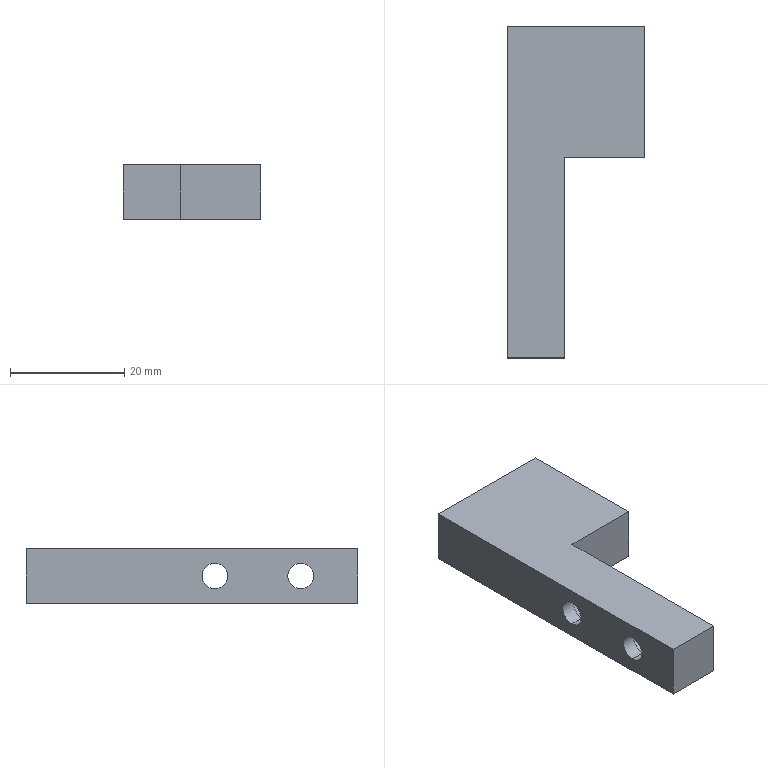Part | STEP file | Rivet air-suction cylinder seat | 1 solid | 26 faces | box 24 x 58 x 9.55 mm | volume 7786 mm3 | cylinder 12 | plane 10 | cone 4 | commonest cylinder face diameters 2.5 x4 4.5 x4 7.5 x4